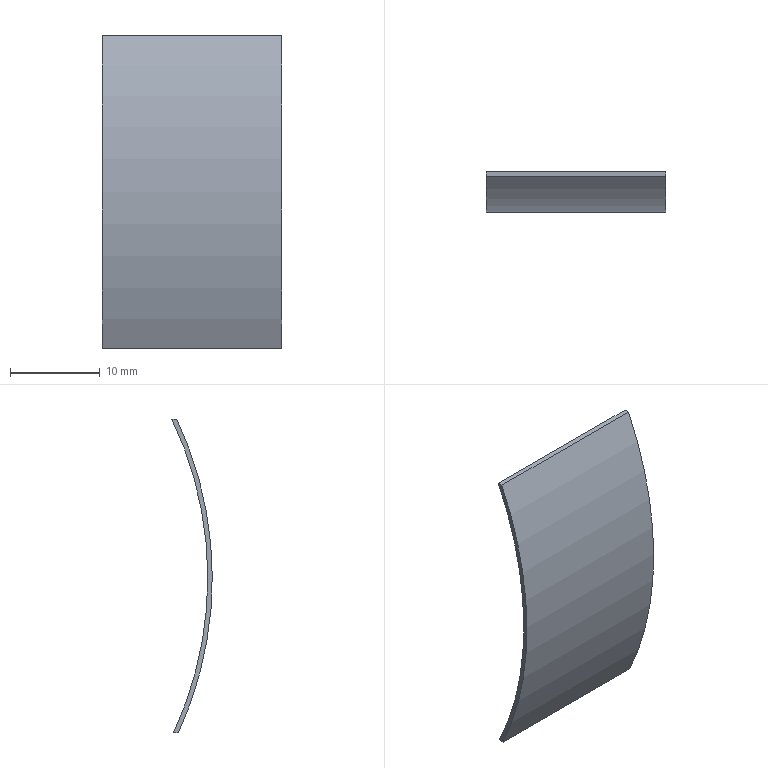Part | STEP file | TQ-DD-1020-BIAOQIAN-001010 | 1 solid | 6 faces | box 20 x 4.519 x 35 mm | volume 361.459 mm3 | plane 4 | cylinder 2 | commonest cylinder face diameters 82 x1 83 x1
STEP:
#1=CARTESIAN_POINT('',(0.,-37.534,17.704));
#2=VERTEX_POINT('',#1);
#3=CARTESIAN_POINT('',(0.,-37.724,-17.296));
#4=VERTEX_POINT('',#3);
#5=CARTESIAN_POINT('',(0.,0.,0.));
#6=DIRECTION('',(1.,0.,0.));
#7=DIRECTION('',(0.,0.,-1.));
#8=AXIS2_PLACEMENT_3D('',#5,#6,#7);
#9=CIRCLE('',#8,41.5);
#10=EDGE_CURVE('',#2,#4,#9,.T.);
#11=ORIENTED_EDGE('',*,*,#10,.T.);
#12=CARTESIAN_POINT('',(20.,-37.724,-17.296));
#13=VERTEX_POINT('',#12);
#14=CARTESIAN_POINT('',(20.,-37.724,-17.296));
#15=DIRECTION('',(-1.,0.,0.));
#16=VECTOR('',#15,1000.);
#17=LINE('',#14,#16);
#18=EDGE_CURVE('',#13,#4,#17,.T.);
#19=ORIENTED_EDGE('',*,*,#18,.F.);
#20=CARTESIAN_POINT('',(20.,-37.534,17.704));
#21=VERTEX_POINT('',#20);
#22=CARTESIAN_POINT('',(20.,0.,0.));
#23=DIRECTION('',(1.,0.,0.));
#24=DIRECTION('',(0.,0.,-1.));
#25=AXIS2_PLACEMENT_3D('',#22,#23,#24);
#26=CIRCLE('',#25,41.5);
#27=EDGE_CURVE('',#21,#13,#26,.T.);
#28=ORIENTED_EDGE('',*,*,#27,.F.);
#29=CARTESIAN_POINT('',(20.,-37.534,17.704));
#30=DIRECTION('',(-1.,0.,0.));
#31=VECTOR('',#30,1000.);
#32=LINE('',#29,#31);
#33=EDGE_CURVE('',#21,#2,#32,.T.);
#34=ORIENTED_EDGE('',*,*,#33,.T.);
#35=EDGE_LOOP('',(#11,#19,#28,#34));
#36=FACE_OUTER_BOUND('',#35,.T.);
#37=CARTESIAN_POINT('',(20.,0.,0.));
#38=DIRECTION('',(-1.,0.,0.));
#39=DIRECTION('',(0.,0.,1.));
#40=AXIS2_PLACEMENT_3D('',#37,#38,#39);
#41=CYLINDRICAL_SURFACE('',#40,41.5);
#42=ADVANCED_FACE('',(#36),#41,.T.);
#43=CARTESIAN_POINT('',(0.,-37.173,-17.296));
#44=VERTEX_POINT('',#43);
#45=CARTESIAN_POINT('',(0.,-37.724,-17.296));
#46=DIRECTION('',(0.,1.,0.));
#47=VECTOR('',#46,1000.);
#48=LINE('',#45,#47);
#49=EDGE_CURVE('',#4,#44,#48,.T.);
#50=ORIENTED_EDGE('',*,*,#49,.T.);
#51=CARTESIAN_POINT('',(20.,-37.173,-17.296));
#52=VERTEX_POINT('',#51);
#53=CARTESIAN_POINT('',(20.,-37.173,-17.296));
#54=DIRECTION('',(-1.,0.,0.));
#55=VECTOR('',#54,1000.);
#56=LINE('',#53,#55);
#57=EDGE_CURVE('',#52,#44,#56,.T.);
#58=ORIENTED_EDGE('',*,*,#57,.F.);
#59=CARTESIAN_POINT('',(20.,-37.724,-17.296));
#60=DIRECTION('',(0.,1.,0.));
#61=VECTOR('',#60,1000.);
#62=LINE('',#59,#61);
#63=EDGE_CURVE('',#13,#52,#62,.T.);
#64=ORIENTED_EDGE('',*,*,#63,.F.);
#65=ORIENTED_EDGE('',*,*,#18,.T.);
#66=EDGE_LOOP('',(#50,#58,#64,#65));
#67=FACE_OUTER_BOUND('',#66,.T.);
#68=CARTESIAN_POINT('',(20.,-37.724,-17.296));
#69=DIRECTION('',(0.,0.,1.));
#70=DIRECTION('',(1.,0.,0.));
#71=AXIS2_PLACEMENT_3D('',#68,#69,#70);
#72=PLANE('',#71);
#73=ADVANCED_FACE('',(#67),#72,.F.);
#74=CARTESIAN_POINT('',(0.,-36.981,17.704));
#75=VERTEX_POINT('',#74);
#76=CARTESIAN_POINT('',(0.,0.,0.));
#77=DIRECTION('',(-1.,0.,0.));
#78=DIRECTION('',(0.,0.,-1.));
#79=AXIS2_PLACEMENT_3D('',#76,#77,#78);
#80=CIRCLE('',#79,41.);
#81=EDGE_CURVE('',#44,#75,#80,.T.);
#82=ORIENTED_EDGE('',*,*,#81,.T.);
#83=CARTESIAN_POINT('',(20.,-36.981,17.704));
#84=VERTEX_POINT('',#83);
#85=CARTESIAN_POINT('',(20.,-36.981,17.704));
#86=DIRECTION('',(-1.,0.,0.));
#87=VECTOR('',#86,1000.);
#88=LINE('',#85,#87);
#89=EDGE_CURVE('',#84,#75,#88,.T.);
#90=ORIENTED_EDGE('',*,*,#89,.F.);
#91=CARTESIAN_POINT('',(20.,0.,0.));
#92=DIRECTION('',(-1.,0.,0.));
#93=DIRECTION('',(0.,0.,-1.));
#94=AXIS2_PLACEMENT_3D('',#91,#92,#93);
#95=CIRCLE('',#94,41.);
#96=EDGE_CURVE('',#52,#84,#95,.T.);
#97=ORIENTED_EDGE('',*,*,#96,.F.);
#98=ORIENTED_EDGE('',*,*,#57,.T.);
#99=EDGE_LOOP('',(#82,#90,#97,#98));
#100=FACE_OUTER_BOUND('',#99,.T.);
#101=CARTESIAN_POINT('',(20.,0.,0.));
#102=DIRECTION('',(-1.,0.,0.));
#103=DIRECTION('',(0.,0.,1.));
#104=AXIS2_PLACEMENT_3D('',#101,#102,#103);
#105=CYLINDRICAL_SURFACE('',#104,41.);
#106=ADVANCED_FACE('',(#100),#105,.F.);
#107=CARTESIAN_POINT('',(0.,-37.534,17.704));
#108=DIRECTION('',(0.,-1.,0.));
#109=VECTOR('',#108,1000.);
#110=LINE('',#107,#109);
#111=EDGE_CURVE('',#75,#2,#110,.T.);
#112=ORIENTED_EDGE('',*,*,#111,.T.);
#113=ORIENTED_EDGE('',*,*,#33,.F.);
#114=CARTESIAN_POINT('',(20.,-37.534,17.704));
#115=DIRECTION('',(0.,-1.,0.));
#116=VECTOR('',#115,1000.);
#117=LINE('',#114,#116);
#118=EDGE_CURVE('',#84,#21,#117,.T.);
#119=ORIENTED_EDGE('',*,*,#118,.F.);
#120=ORIENTED_EDGE('',*,*,#89,.T.);
#121=EDGE_LOOP('',(#112,#113,#119,#120));
#122=FACE_OUTER_BOUND('',#121,.T.);
#123=CARTESIAN_POINT('',(20.,-37.534,17.704));
#124=DIRECTION('',(0.,0.,-1.));
#125=DIRECTION('',(-1.,0.,0.));
#126=AXIS2_PLACEMENT_3D('',#123,#124,#125);
#127=PLANE('',#126);
#128=ADVANCED_FACE('',(#122),#127,.F.);
#129=ORIENTED_EDGE('',*,*,#27,.T.);
#130=ORIENTED_EDGE('',*,*,#63,.T.);
#131=ORIENTED_EDGE('',*,*,#96,.T.);
#132=ORIENTED_EDGE('',*,*,#118,.T.);
#133=EDGE_LOOP('',(#129,#130,#131,#132));
#134=FACE_OUTER_BOUND('',#133,.T.);
#135=CARTESIAN_POINT('',(20.,0.,0.));
#136=DIRECTION('',(1.,0.,0.));
#137=DIRECTION('',(0.,0.,-1.));
#138=AXIS2_PLACEMENT_3D('',#135,#136,#137);
#139=PLANE('',#138);
#140=ADVANCED_FACE('',(#134),#139,.T.);
#141=ORIENTED_EDGE('',*,*,#10,.F.);
#142=ORIENTED_EDGE('',*,*,#111,.F.);
#143=ORIENTED_EDGE('',*,*,#81,.F.);
#144=ORIENTED_EDGE('',*,*,#49,.F.);
#145=EDGE_LOOP('',(#141,#142,#143,#144));
#146=FACE_OUTER_BOUND('',#145,.T.);
#147=CARTESIAN_POINT('',(0.,0.,0.));
#148=DIRECTION('',(1.,0.,0.));
#149=DIRECTION('',(0.,0.,-1.));
#150=AXIS2_PLACEMENT_3D('',#147,#148,#149);
#151=PLANE('',#150);
#152=ADVANCED_FACE('',(#146),#151,.F.);
#153=CLOSED_SHELL('',(#42,#73,#106,#128,#140,#152));
#154=MANIFOLD_SOLID_BREP('',#153);
#155=CARTESIAN_POINT('',(0.,0.,0.));
#156=DIRECTION('',(0.,0.,1.));
#157=DIRECTION('',(1.,0.,0.));
#158=AXIS2_PLACEMENT_3D('',#155,#156,#157);
#159=(LENGTH_UNIT()NAMED_UNIT(*)SI_UNIT(.MILLI.,.METRE.));
#160=UNCERTAINTY_MEASURE_WITH_UNIT(LENGTH_MEASURE(0.00001),#159,'','');
#161=(NAMED_UNIT(*)PLANE_ANGLE_UNIT()SI_UNIT($,.RADIAN.));
#162=(NAMED_UNIT(*)SI_UNIT($,.STERADIAN.)SOLID_ANGLE_UNIT());
#163=(GEOMETRIC_REPRESENTATION_CONTEXT(3)GLOBAL_UNCERTAINTY_ASSIGNED_CONTEXT((#160))GLOBAL_UNIT_ASSIGNED_CONTEXT((#159,#161,#162))REPRESENTATION_CONTEXT('',''));
#164=ADVANCED_BREP_SHAPE_REPRESENTATION('',(#154,#158),#163);